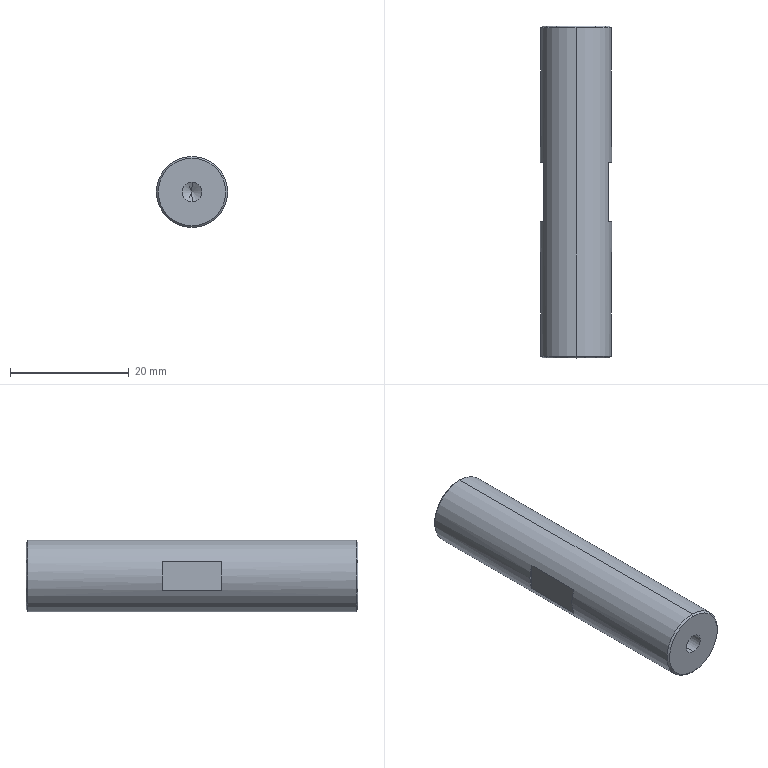Part | STEP file | ND25021-01-JDKM-09B-TL | 1 solid | 22 faces | box 12 x 56 x 12 mm | volume 6119 mm3 | cone 8 | plane 8 | cylinder 6 | commonest cylinder face diameters 3.3 x4 12 x2
STEP:
#1=CARTESIAN_POINT('',(0.,0.,0.));
#2=DIRECTION('',(0.,0.,1.));
#3=DIRECTION('',(1.,0.,0.));
#4=AXIS2_PLACEMENT_3D('',#1,#2,#3);
#5=CARTESIAN_POINT('',(0.,-28.,-5.7));
#6=VERTEX_POINT('',#5);
#7=CARTESIAN_POINT('',(0.,-28.,5.7));
#8=VERTEX_POINT('',#7);
#9=CARTESIAN_POINT('',(0.,-28.,0.));
#10=DIRECTION('',(0.,-1.,0.));
#11=DIRECTION('',(0.,0.,1.));
#12=AXIS2_PLACEMENT_3D('',#9,#10,#11);
#13=CIRCLE('',#12,5.7);
#14=CARTESIAN_POINT('',(0.,-27.7,0.));
#15=DIRECTION('',(0.,1.,0.));
#16=DIRECTION('',(0.,0.,1.));
#17=AXIS2_PLACEMENT_3D('',#14,#15,#16);
#18=CONICAL_SURFACE('',#17,6.,0.7854);
#19=CARTESIAN_POINT('',(6.283,-0.3));
#20=DIRECTION('',(-1.,0.));
#21=VECTOR('',#20,1.);
#22=LINE('',#19,#21);
#23=(GEOMETRIC_REPRESENTATION_CONTEXT(2)PARAMETRIC_REPRESENTATION_CONTEXT()REPRESENTATION_CONTEXT('',''));
#24=DEFINITIONAL_REPRESENTATION('',(#22),#23);
#25=PCURVE('',#18,#24);
#26=CARTESIAN_POINT('',(0.,-28.,0.));
#27=DIRECTION('',(0.,1.,0.));
#28=DIRECTION('',(0.,0.,1.));
#29=AXIS2_PLACEMENT_3D('',#26,#27,#28);
#30=PLANE('',#29);
#31=CARTESIAN_POINT('',(5.7,0.));
#32=CARTESIAN_POINT('',(5.7,-9.873));
#33=CARTESIAN_POINT('',(-2.85,-4.936));
#34=CARTESIAN_POINT('',(-11.4,0.));
#35=CARTESIAN_POINT('',(-2.85,4.936));
#36=CARTESIAN_POINT('',(5.7,9.873));
#37=CARTESIAN_POINT('',(5.7,0.));
#38=(BOUNDED_CURVE()B_SPLINE_CURVE(2,(#31,#32,#33,#34,#35,#36,#37),.UNSPECIFIED.,.T.,.F.)B_SPLINE_CURVE_WITH_KNOTS((1,2,2,2,2,1),(-2.094,0.,2.094,4.189,6.283,8.378),.UNSPECIFIED.)CURVE()GEOMETRIC_REPRESENTATION_ITEM()RATIONAL_B_SPLINE_CURVE((1.,0.5,1.,0.5,1.,0.5,1.))REPRESENTATION_ITEM(''));
#39=(GEOMETRIC_REPRESENTATION_CONTEXT(2)PARAMETRIC_REPRESENTATION_CONTEXT()REPRESENTATION_CONTEXT('',''));
#40=DEFINITIONAL_REPRESENTATION('',(#38),#39);
#41=PCURVE('',#30,#40);
#42=SURFACE_CURVE('',#13,(#25,#41),.PCURVE_S1.);
#43=EDGE_CURVE('',#6,#8,#42,.T.);
#44=ORIENTED_EDGE('',*,*,#43,.F.);
#45=CARTESIAN_POINT('',(0.,-27.7,-6.));
#46=VERTEX_POINT('',#45);
#47=CARTESIAN_POINT('',(0.,-27.7,-6.));
#48=DIRECTION('',(0.,0.7071,-0.7071));
#49=VECTOR('',#48,1.);
#50=LINE('',#47,#49);
#51=CARTESIAN_POINT('',(3.142,0.));
#52=DIRECTION('',(0.,1.));
#53=VECTOR('',#52,1.);
#54=LINE('',#51,#53);
#55=(GEOMETRIC_REPRESENTATION_CONTEXT(2)PARAMETRIC_REPRESENTATION_CONTEXT()REPRESENTATION_CONTEXT('',''));
#56=DEFINITIONAL_REPRESENTATION('',(#54),#55);
#57=PCURVE('',#18,#56);
#58=CARTESIAN_POINT('',(0.,-27.7,0.));
#59=DIRECTION('',(0.,1.,0.));
#60=DIRECTION('',(0.,0.,1.));
#61=AXIS2_PLACEMENT_3D('',#58,#59,#60);
#62=CONICAL_SURFACE('',#61,6.,0.7854);
#63=CARTESIAN_POINT('',(3.142,0.));
#64=DIRECTION('',(0.,1.));
#65=VECTOR('',#64,1.);
#66=LINE('',#63,#65);
#67=(GEOMETRIC_REPRESENTATION_CONTEXT(2)PARAMETRIC_REPRESENTATION_CONTEXT()REPRESENTATION_CONTEXT('',''));
#68=DEFINITIONAL_REPRESENTATION('',(#66),#67);
#69=PCURVE('',#62,#68);
#70=SURFACE_CURVE('',#50,(#57,#69),.PCURVE_S1.);
#71=EDGE_CURVE('',#6,#46,#70,.T.);
#72=ORIENTED_EDGE('',*,*,#71,.T.);
#73=CARTESIAN_POINT('',(0.,-27.7,6.));
#74=VERTEX_POINT('',#73);
#75=CARTESIAN_POINT('',(0.,-27.7,0.));
#76=DIRECTION('',(0.,1.,0.));
#77=DIRECTION('',(0.,0.,1.));
#78=AXIS2_PLACEMENT_3D('',#75,#76,#77);
#79=CIRCLE('',#78,6.);
#80=CARTESIAN_POINT('',(0.,0.));
#81=DIRECTION('',(1.,0.));
#82=VECTOR('',#81,1.);
#83=LINE('',#80,#82);
#84=(GEOMETRIC_REPRESENTATION_CONTEXT(2)PARAMETRIC_REPRESENTATION_CONTEXT()REPRESENTATION_CONTEXT('',''));
#85=DEFINITIONAL_REPRESENTATION('',(#83),#84);
#86=PCURVE('',#18,#85);
#87=CARTESIAN_POINT('',(0.,28.,0.));
#88=DIRECTION('',(0.,-1.,0.));
#89=DIRECTION('',(0.,0.,-1.));
#90=AXIS2_PLACEMENT_3D('',#87,#88,#89);
#91=CYLINDRICAL_SURFACE('',#90,6.);
#92=CARTESIAN_POINT('',(3.142,55.7));
#93=DIRECTION('',(-1.,0.));
#94=VECTOR('',#93,1.);
#95=LINE('',#92,#94);
#96=(GEOMETRIC_REPRESENTATION_CONTEXT(2)PARAMETRIC_REPRESENTATION_CONTEXT()REPRESENTATION_CONTEXT('',''));
#97=DEFINITIONAL_REPRESENTATION('',(#95),#96);
#98=PCURVE('',#91,#97);
#99=SURFACE_CURVE('',#79,(#86,#98),.PCURVE_S1.);
#100=EDGE_CURVE('',#74,#46,#99,.T.);
#101=ORIENTED_EDGE('',*,*,#100,.F.);
#102=CARTESIAN_POINT('',(0.,-27.7,6.));
#103=DIRECTION('',(0.,0.7071,0.7071));
#104=VECTOR('',#103,1.);
#105=LINE('',#102,#104);
#106=CARTESIAN_POINT('',(0.,0.));
#107=DIRECTION('',(0.,1.));
#108=VECTOR('',#107,1.);
#109=LINE('',#106,#108);
#110=(GEOMETRIC_REPRESENTATION_CONTEXT(2)PARAMETRIC_REPRESENTATION_CONTEXT()REPRESENTATION_CONTEXT('',''));
#111=DEFINITIONAL_REPRESENTATION('',(#109),#110);
#112=PCURVE('',#18,#111);
#113=CARTESIAN_POINT('',(6.283,0.));
#114=DIRECTION('',(0.,1.));
#115=VECTOR('',#114,1.);
#116=LINE('',#113,#115);
#117=(GEOMETRIC_REPRESENTATION_CONTEXT(2)PARAMETRIC_REPRESENTATION_CONTEXT()REPRESENTATION_CONTEXT('',''));
#118=DEFINITIONAL_REPRESENTATION('',(#116),#117);
#119=PCURVE('',#62,#118);
#120=SURFACE_CURVE('',#105,(#112,#119),.PCURVE_S1.);
#121=EDGE_CURVE('',#8,#74,#120,.T.);
#122=ORIENTED_EDGE('',*,*,#121,.F.);
#123=EDGE_LOOP('',(#44,#72,#101,#122));
#124=FACE_BOUND('',#123,.T.);
#125=ADVANCED_FACE('',(#124),#18,.T.);
#126=CARTESIAN_POINT('',(0.,28.,5.7));
#127=VERTEX_POINT('',#126);
#128=CARTESIAN_POINT('',(0.,28.,-5.7));
#129=VERTEX_POINT('',#128);
#130=CARTESIAN_POINT('',(0.,28.,0.));
#131=DIRECTION('',(0.,1.,0.));
#132=DIRECTION('',(0.,0.,1.));
#133=AXIS2_PLACEMENT_3D('',#130,#131,#132);
#134=CIRCLE('',#133,5.7);
#135=CARTESIAN_POINT('',(0.,28.,0.));
#136=DIRECTION('',(0.,-1.,0.));
#137=DIRECTION('',(0.,0.,-1.));
#138=AXIS2_PLACEMENT_3D('',#135,#136,#137);
#139=CONICAL_SURFACE('',#138,5.7,0.7854);
#140=CARTESIAN_POINT('',(3.142,0.));
#141=DIRECTION('',(-1.,0.));
#142=VECTOR('',#141,1.);
#143=LINE('',#140,#142);
#144=(GEOMETRIC_REPRESENTATION_CONTEXT(2)PARAMETRIC_REPRESENTATION_CONTEXT()REPRESENTATION_CONTEXT('',''));
#145=DEFINITIONAL_REPRESENTATION('',(#143),#144);
#146=PCURVE('',#139,#145);
#147=CARTESIAN_POINT('',(0.,28.,0.));
#148=DIRECTION('',(0.,1.,0.));
#149=DIRECTION('',(0.,0.,1.));
#150=AXIS2_PLACEMENT_3D('',#147,#148,#149);
#151=PLANE('',#150);
#152=CARTESIAN_POINT('',(0.,0.));
#153=DIRECTION('',(1.,0.));
#154=AXIS2_PLACEMENT_2D('',#152,#153);
#155=CIRCLE('',#154,5.7);
#156=(GEOMETRIC_REPRESENTATION_CONTEXT(2)PARAMETRIC_REPRESENTATION_CONTEXT()REPRESENTATION_CONTEXT('',''));
#157=DEFINITIONAL_REPRESENTATION('',(#155),#156);
#158=PCURVE('',#151,#157);
#159=SURFACE_CURVE('',#134,(#146,#158),.PCURVE_S1.);
#160=EDGE_CURVE('',#127,#129,#159,.T.);
#161=ORIENTED_EDGE('',*,*,#160,.F.);
#162=CARTESIAN_POINT('',(0.,27.7,6.));
#163=VERTEX_POINT('',#162);
#164=CARTESIAN_POINT('',(0.,28.,5.7));
#165=DIRECTION('',(0.,-0.7071,0.7071));
#166=VECTOR('',#165,1.);
#167=LINE('',#164,#166);
#168=CARTESIAN_POINT('',(3.142,0.));
#169=DIRECTION('',(0.,1.));
#170=VECTOR('',#169,1.);
#171=LINE('',#168,#170);
#172=(GEOMETRIC_REPRESENTATION_CONTEXT(2)PARAMETRIC_REPRESENTATION_CONTEXT()REPRESENTATION_CONTEXT('',''));
#173=DEFINITIONAL_REPRESENTATION('',(#171),#172);
#174=PCURVE('',#139,#173);
#175=CARTESIAN_POINT('',(0.,28.,0.));
#176=DIRECTION('',(0.,-1.,0.));
#177=DIRECTION('',(0.,0.,-1.));
#178=AXIS2_PLACEMENT_3D('',#175,#176,#177);
#179=CONICAL_SURFACE('',#178,5.7,0.7854);
#180=CARTESIAN_POINT('',(3.142,0.));
#181=DIRECTION('',(0.,1.));
#182=VECTOR('',#181,1.);
#183=LINE('',#180,#182);
#184=(GEOMETRIC_REPRESENTATION_CONTEXT(2)PARAMETRIC_REPRESENTATION_CONTEXT()REPRESENTATION_CONTEXT('',''));
#185=DEFINITIONAL_REPRESENTATION('',(#183),#184);
#186=PCURVE('',#179,#185);
#187=SURFACE_CURVE('',#167,(#174,#186),.PCURVE_S1.);
#188=EDGE_CURVE('',#127,#163,#187,.T.);
#189=ORIENTED_EDGE('',*,*,#188,.T.);
#190=CARTESIAN_POINT('',(0.,27.7,-6.));
#191=VERTEX_POINT('',#190);
#192=CARTESIAN_POINT('',(0.,27.7,0.));
#193=DIRECTION('',(0.,-1.,0.));
#194=DIRECTION('',(0.,0.,1.));
#195=AXIS2_PLACEMENT_3D('',#192,#193,#194);
#196=CIRCLE('',#195,6.);
#197=CARTESIAN_POINT('',(-3.142,0.3));
#198=DIRECTION('',(1.,0.));
#199=VECTOR('',#198,1.);
#200=LINE('',#197,#199);
#201=(GEOMETRIC_REPRESENTATION_CONTEXT(2)PARAMETRIC_REPRESENTATION_CONTEXT()REPRESENTATION_CONTEXT('',''));
#202=DEFINITIONAL_REPRESENTATION('',(#200),#201);
#203=PCURVE('',#139,#202);
#204=CARTESIAN_POINT('',(-3.142,0.3));
#205=DIRECTION('',(1.,0.));
#206=VECTOR('',#205,1.);
#207=LINE('',#204,#206);
#208=(GEOMETRIC_REPRESENTATION_CONTEXT(2)PARAMETRIC_REPRESENTATION_CONTEXT()REPRESENTATION_CONTEXT('',''));
#209=DEFINITIONAL_REPRESENTATION('',(#207),#208);
#210=PCURVE('',#91,#209);
#211=SURFACE_CURVE('',#196,(#203,#210),.PCURVE_S1.);
#212=EDGE_CURVE('',#191,#163,#211,.T.);
#213=ORIENTED_EDGE('',*,*,#212,.F.);
#214=CARTESIAN_POINT('',(0.,28.,-5.7));
#215=DIRECTION('',(0.,-0.7071,-0.7071));
#216=VECTOR('',#215,1.);
#217=LINE('',#214,#216);
#218=CARTESIAN_POINT('',(0.,0.));
#219=DIRECTION('',(0.,1.));
#220=VECTOR('',#219,1.);
#221=LINE('',#218,#220);
#222=(GEOMETRIC_REPRESENTATION_CONTEXT(2)PARAMETRIC_REPRESENTATION_CONTEXT()REPRESENTATION_CONTEXT('',''));
#223=DEFINITIONAL_REPRESENTATION('',(#221),#222);
#224=PCURVE('',#139,#223);
#225=CARTESIAN_POINT('',(6.283,0.));
#226=DIRECTION('',(0.,1.));
#227=VECTOR('',#226,1.);
#228=LINE('',#225,#227);
#229=(GEOMETRIC_REPRESENTATION_CONTEXT(2)PARAMETRIC_REPRESENTATION_CONTEXT()REPRESENTATION_CONTEXT('',''));
#230=DEFINITIONAL_REPRESENTATION('',(#228),#229);
#231=PCURVE('',#179,#230);
#232=SURFACE_CURVE('',#217,(#224,#231),.PCURVE_S1.);
#233=EDGE_CURVE('',#129,#191,#232,.T.);
#234=ORIENTED_EDGE('',*,*,#233,.F.);
#235=EDGE_LOOP('',(#161,#189,#213,#234));
#236=FACE_BOUND('',#235,.T.);
#237=ADVANCED_FACE('',(#236),#139,.T.);
#238=CARTESIAN_POINT('',(0.,-17.9,-1.65));
#239=VERTEX_POINT('',#238);
#240=CARTESIAN_POINT('',(0.,-28.,-1.65));
#241=VERTEX_POINT('',#240);
#242=CARTESIAN_POINT('',(0.,-28.,-1.65));
#243=DIRECTION('',(0.,-1.,0.));
#244=VECTOR('',#243,1.);
#245=LINE('',#242,#244);
#246=CARTESIAN_POINT('',(0.,-28.,0.));
#247=DIRECTION('',(0.,-1.,0.));
#248=DIRECTION('',(0.,0.,-1.));
#249=AXIS2_PLACEMENT_3D('',#246,#247,#248);
#250=CYLINDRICAL_SURFACE('',#249,1.65);
#251=CARTESIAN_POINT('',(6.283,0.));
#252=DIRECTION('',(0.,1.));
#253=VECTOR('',#252,1.);
#254=LINE('',#251,#253);
#255=(GEOMETRIC_REPRESENTATION_CONTEXT(2)PARAMETRIC_REPRESENTATION_CONTEXT()REPRESENTATION_CONTEXT('',''));
#256=DEFINITIONAL_REPRESENTATION('',(#254),#255);
#257=PCURVE('',#250,#256);
#258=CARTESIAN_POINT('',(0.,-28.,0.));
#259=DIRECTION('',(0.,-1.,0.));
#260=DIRECTION('',(0.,0.,-1.));
#261=AXIS2_PLACEMENT_3D('',#258,#259,#260);
#262=CYLINDRICAL_SURFACE('',#261,1.65);
#263=CARTESIAN_POINT('',(0.,0.));
#264=DIRECTION('',(0.,1.));
#265=VECTOR('',#264,1.);
#266=LINE('',#263,#265);
#267=(GEOMETRIC_REPRESENTATION_CONTEXT(2)PARAMETRIC_REPRESENTATION_CONTEXT()REPRESENTATION_CONTEXT('',''));
#268=DEFINITIONAL_REPRESENTATION('',(#266),#267);
#269=PCURVE('',#262,#268);
#270=SURFACE_CURVE('',#245,(#257,#269),.PCURVE_S1.);
#271=EDGE_CURVE('',#239,#241,#270,.T.);
#272=ORIENTED_EDGE('',*,*,#271,.T.);
#273=CARTESIAN_POINT('',(0.,-28.,1.65));
#274=VERTEX_POINT('',#273);
#275=CARTESIAN_POINT('',(0.,-28.,0.));
#276=DIRECTION('',(0.,-1.,0.));
#277=DIRECTION('',(0.,0.,-1.));
#278=AXIS2_PLACEMENT_3D('',#275,#276,#277);
#279=CIRCLE('',#278,1.65);
#280=CARTESIAN_POINT('',(0.,0.));
#281=DIRECTION('',(1.,0.));
#282=VECTOR('',#281,1.);
#283=LINE('',#280,#282);
#284=(GEOMETRIC_REPRESENTATION_CONTEXT(2)PARAMETRIC_REPRESENTATION_CONTEXT()REPRESENTATION_CONTEXT('',''));
#285=DEFINITIONAL_REPRESENTATION('',(#283),#284);
#286=PCURVE('',#250,#285);
#287=CARTESIAN_POINT('',(-1.65,0.));
#288=CARTESIAN_POINT('',(-1.65,2.858));
#289=CARTESIAN_POINT('',(0.825,1.429));
#290=CARTESIAN_POINT('',(3.3,0.));
#291=CARTESIAN_POINT('',(0.825,-1.429));
#292=CARTESIAN_POINT('',(-1.65,-2.858));
#293=CARTESIAN_POINT('',(-1.65,0.));
#294=(BOUNDED_CURVE()B_SPLINE_CURVE(2,(#287,#288,#289,#290,#291,#292,#293),.UNSPECIFIED.,.T.,.F.)B_SPLINE_CURVE_WITH_KNOTS((1,2,2,2,2,1),(-2.094,0.,2.094,4.189,6.283,8.378),.UNSPECIFIED.)CURVE()GEOMETRIC_REPRESENTATION_ITEM()RATIONAL_B_SPLINE_CURVE((1.,0.5,1.,0.5,1.,0.5,1.))REPRESENTATION_ITEM(''));
#295=(GEOMETRIC_REPRESENTATION_CONTEXT(2)PARAMETRIC_REPRESENTATION_CONTEXT()REPRESENTATION_CONTEXT('',''));
#296=DEFINITIONAL_REPRESENTATION('',(#294),#295);
#297=PCURVE('',#30,#296);
#298=SURFACE_CURVE('',#279,(#286,#297),.PCURVE_S1.);
#299=EDGE_CURVE('',#274,#241,#298,.T.);
#300=ORIENTED_EDGE('',*,*,#299,.F.);
#301=CARTESIAN_POINT('',(0.,-17.9,1.65));
#302=VERTEX_POINT('',#301);
#303=CARTESIAN_POINT('',(0.,-28.,1.65));
#304=DIRECTION('',(0.,-1.,0.));
#305=VECTOR('',#304,1.);
#306=LINE('',#303,#305);
#307=CARTESIAN_POINT('',(3.142,0.));
#308=DIRECTION('',(0.,1.));
#309=VECTOR('',#308,1.);
#310=LINE('',#307,#309);
#311=(GEOMETRIC_REPRESENTATION_CONTEXT(2)PARAMETRIC_REPRESENTATION_CONTEXT()REPRESENTATION_CONTEXT('',''));
#312=DEFINITIONAL_REPRESENTATION('',(#310),#311);
#313=PCURVE('',#250,#312);
#314=CARTESIAN_POINT('',(3.142,0.));
#315=DIRECTION('',(0.,1.));
#316=VECTOR('',#315,1.);
#317=LINE('',#314,#316);
#318=(GEOMETRIC_REPRESENTATION_CONTEXT(2)PARAMETRIC_REPRESENTATION_CONTEXT()REPRESENTATION_CONTEXT('',''));
#319=DEFINITIONAL_REPRESENTATION('',(#317),#318);
#320=PCURVE('',#262,#319);
#321=SURFACE_CURVE('',#306,(#313,#320),.PCURVE_S1.);
#322=EDGE_CURVE('',#302,#274,#321,.T.);
#323=ORIENTED_EDGE('',*,*,#322,.F.);
#324=CARTESIAN_POINT('',(0.,-17.9,0.));
#325=DIRECTION('',(0.,-1.,0.));
#326=DIRECTION('',(0.,0.,-1.));
#327=AXIS2_PLACEMENT_3D('',#324,#325,#326);
#328=CIRCLE('',#327,1.65);
#329=CARTESIAN_POINT('',(0.,-10.1));
#330=DIRECTION('',(1.,0.));
#331=VECTOR('',#330,1.);
#332=LINE('',#329,#331);
#333=(GEOMETRIC_REPRESENTATION_CONTEXT(2)PARAMETRIC_REPRESENTATION_CONTEXT()REPRESENTATION_CONTEXT('',''));
#334=DEFINITIONAL_REPRESENTATION('',(#332),#333);
#335=PCURVE('',#250,#334);
#336=CARTESIAN_POINT('',(0.,-17.9,0.));
#337=DIRECTION('',(0.,-1.,0.));
#338=DIRECTION('',(0.,0.,-1.));
#339=AXIS2_PLACEMENT_3D('',#336,#337,#338);
#340=CONICAL_SURFACE('',#339,1.65,1.03);
#341=CARTESIAN_POINT('',(0.,0.));
#342=DIRECTION('',(1.,0.));
#343=VECTOR('',#342,1.);
#344=LINE('',#341,#343);
#345=(GEOMETRIC_REPRESENTATION_CONTEXT(2)PARAMETRIC_REPRESENTATION_CONTEXT()REPRESENTATION_CONTEXT('',''));
#346=DEFINITIONAL_REPRESENTATION('',(#344),#345);
#347=PCURVE('',#340,#346);
#348=SURFACE_CURVE('',#328,(#335,#347),.PCURVE_S1.);
#349=EDGE_CURVE('',#302,#239,#348,.T.);
#350=ORIENTED_EDGE('',*,*,#349,.T.);
#351=EDGE_LOOP('',(#272,#300,#323,#350));
#352=FACE_BOUND('',#351,.F.);
#353=ADVANCED_FACE('',(#352),#250,.F.);
#354=ORIENTED_EDGE('',*,*,#349,.F.);
#355=CARTESIAN_POINT('',(0.,-16.909,0.));
#356=VERTEX_POINT('',#355);
#357=CARTESIAN_POINT('',(0.,-17.9,1.65));
#358=DIRECTION('',(0.,-0.515,0.8572));
#359=VECTOR('',#358,1.);
#360=LINE('',#357,#359);
#361=CARTESIAN_POINT('',(3.142,-0.9914));
#362=CARTESIAN_POINT('',(3.142,-0.9764));
#363=CARTESIAN_POINT('',(3.142,-0.9464));
#364=CARTESIAN_POINT('',(3.142,-0.9013));
#365=CARTESIAN_POINT('',(3.142,-0.8562));
#366=CARTESIAN_POINT('',(3.142,-0.8112));
#367=CARTESIAN_POINT('',(3.142,-0.7661));
#368=CARTESIAN_POINT('',(3.142,-0.721));
#369=CARTESIAN_POINT('',(3.142,-0.676));
#370=CARTESIAN_POINT('',(3.142,-0.6309));
#371=CARTESIAN_POINT('',(3.142,-0.5858));
#372=CARTESIAN_POINT('',(3.142,-0.5408));
#373=CARTESIAN_POINT('',(3.142,-0.4957));
#374=CARTESIAN_POINT('',(3.142,-0.4506));
#375=CARTESIAN_POINT('',(3.142,-0.4056));
#376=CARTESIAN_POINT('',(3.142,-0.3605));
#377=CARTESIAN_POINT('',(3.142,-0.3155));
#378=CARTESIAN_POINT('',(3.142,-0.2704));
#379=CARTESIAN_POINT('',(3.142,-0.2253));
#380=CARTESIAN_POINT('',(3.142,-0.1803));
#381=CARTESIAN_POINT('',(3.142,-0.1352));
#382=CARTESIAN_POINT('',(3.142,-0.09013));
#383=CARTESIAN_POINT('',(3.142,-0.04506));
#384=CARTESIAN_POINT('',(3.142,-0.01502));
#385=CARTESIAN_POINT('',(3.142,0.));
#386=B_SPLINE_CURVE_WITH_KNOTS('',3,(#361,#362,#363,#364,#365,#366,#367,#368,#369,#370,#371,#372,#373,#374,#375,#376,#377,#378,#379,#380,#381,#382,#383,#384,#385),.UNSPECIFIED.,.F.,.F.,(4,1,1,1,1,1,1,1,1,1,1,1,1,1,1,1,1,1,1,1,1,1,4),(-1.925,-1.837,-1.75,-1.662,-1.575,-1.487,-1.4,-1.312,-1.225,-1.137,-1.05,-0.9625,-0.875,-0.7875,-0.7,-0.6125,-0.525,-0.4375,-0.35,-0.2625,-0.175,-0.0875,0.),.UNSPECIFIED.);
#387=(GEOMETRIC_REPRESENTATION_CONTEXT(2)PARAMETRIC_REPRESENTATION_CONTEXT()REPRESENTATION_CONTEXT('',''));
#388=DEFINITIONAL_REPRESENTATION('',(#386),#387);
#389=PCURVE('',#340,#388);
#390=CARTESIAN_POINT('',(0.,-17.9,0.));
#391=DIRECTION('',(0.,-1.,0.));
#392=DIRECTION('',(0.,0.,-1.));
#393=AXIS2_PLACEMENT_3D('',#390,#391,#392);
#394=CONICAL_SURFACE('',#393,1.65,1.03);
#395=CARTESIAN_POINT('',(3.142,-0.9914));
#396=CARTESIAN_POINT('',(3.142,-0.9764));
#397=CARTESIAN_POINT('',(3.142,-0.9464));
#398=CARTESIAN_POINT('',(3.142,-0.9013));
#399=CARTESIAN_POINT('',(3.142,-0.8562));
#400=CARTESIAN_POINT('',(3.142,-0.8112));
#401=CARTESIAN_POINT('',(3.142,-0.7661));
#402=CARTESIAN_POINT('',(3.142,-0.721));
#403=CARTESIAN_POINT('',(3.142,-0.676));
#404=CARTESIAN_POINT('',(3.142,-0.6309));
#405=CARTESIAN_POINT('',(3.142,-0.5858));
#406=CARTESIAN_POINT('',(3.142,-0.5408));
#407=CARTESIAN_POINT('',(3.142,-0.4957));
#408=CARTESIAN_POINT('',(3.142,-0.4506));
#409=CARTESIAN_POINT('',(3.142,-0.4056));
#410=CARTESIAN_POINT('',(3.142,-0.3605));
#411=CARTESIAN_POINT('',(3.142,-0.3155));
#412=CARTESIAN_POINT('',(3.142,-0.2704));
#413=CARTESIAN_POINT('',(3.142,-0.2253));
#414=CARTESIAN_POINT('',(3.142,-0.1803));
#415=CARTESIAN_POINT('',(3.142,-0.1352));
#416=CARTESIAN_POINT('',(3.142,-0.09013));
#417=CARTESIAN_POINT('',(3.142,-0.04506));
#418=CARTESIAN_POINT('',(3.142,-0.01502));
#419=CARTESIAN_POINT('',(3.142,0.));
#420=B_SPLINE_CURVE_WITH_KNOTS('',3,(#395,#396,#397,#398,#399,#400,#401,#402,#403,#404,#405,#406,#407,#408,#409,#410,#411,#412,#413,#414,#415,#416,#417,#418,#419),.UNSPECIFIED.,.F.,.F.,(4,1,1,1,1,1,1,1,1,1,1,1,1,1,1,1,1,1,1,1,1,1,4),(-1.925,-1.837,-1.75,-1.662,-1.575,-1.487,-1.4,-1.312,-1.225,-1.137,-1.05,-0.9625,-0.875,-0.7875,-0.7,-0.6125,-0.525,-0.4375,-0.35,-0.2625,-0.175,-0.0875,0.),.UNSPECIFIED.);
#421=(GEOMETRIC_REPRESENTATION_CONTEXT(2)PARAMETRIC_REPRESENTATION_CONTEXT()REPRESENTATION_CONTEXT('',''));
#422=DEFINITIONAL_REPRESENTATION('',(#420),#421);
#423=PCURVE('',#394,#422);
#424=SURFACE_CURVE('',#360,(#389,#423),.PCURVE_S1.);
#425=EDGE_CURVE('',#356,#302,#424,.T.);
#426=ORIENTED_EDGE('',*,*,#425,.F.);
#427=CARTESIAN_POINT('',(0.,-17.9,-1.65));
#428=DIRECTION('',(0.,-0.515,-0.8572));
#429=VECTOR('',#428,1.);
#430=LINE('',#427,#429);
#431=CARTESIAN_POINT('',(6.283,-0.9914));
#432=CARTESIAN_POINT('',(6.283,-0.9764));
#433=CARTESIAN_POINT('',(6.283,-0.9464));
#434=CARTESIAN_POINT('',(6.283,-0.9013));
#435=CARTESIAN_POINT('',(6.283,-0.8562));
#436=CARTESIAN_POINT('',(6.283,-0.8112));
#437=CARTESIAN_POINT('',(6.283,-0.7661));
#438=CARTESIAN_POINT('',(6.283,-0.721));
#439=CARTESIAN_POINT('',(6.283,-0.676));
#440=CARTESIAN_POINT('',(6.283,-0.6309));
#441=CARTESIAN_POINT('',(6.283,-0.5858));
#442=CARTESIAN_POINT('',(6.283,-0.5408));
#443=CARTESIAN_POINT('',(6.283,-0.4957));
#444=CARTESIAN_POINT('',(6.283,-0.4506));
#445=CARTESIAN_POINT('',(6.283,-0.4056));
#446=CARTESIAN_POINT('',(6.283,-0.3605));
#447=CARTESIAN_POINT('',(6.283,-0.3155));
#448=CARTESIAN_POINT('',(6.283,-0.2704));
#449=CARTESIAN_POINT('',(6.283,-0.2253));
#450=CARTESIAN_POINT('',(6.283,-0.1803));
#451=CARTESIAN_POINT('',(6.283,-0.1352));
#452=CARTESIAN_POINT('',(6.283,-0.09013));
#453=CARTESIAN_POINT('',(6.283,-0.04506));
#454=CARTESIAN_POINT('',(6.283,-0.01502));
#455=CARTESIAN_POINT('',(6.283,0.));
#456=B_SPLINE_CURVE_WITH_KNOTS('',3,(#431,#432,#433,#434,#435,#436,#437,#438,#439,#440,#441,#442,#443,#444,#445,#446,#447,#448,#449,#450,#451,#452,#453,#454,#455),.UNSPECIFIED.,.F.,.F.,(4,1,1,1,1,1,1,1,1,1,1,1,1,1,1,1,1,1,1,1,1,1,4),(-1.925,-1.837,-1.75,-1.662,-1.575,-1.487,-1.4,-1.312,-1.225,-1.137,-1.05,-0.9625,-0.875,-0.7875,-0.7,-0.6125,-0.525,-0.4375,-0.35,-0.2625,-0.175,-0.0875,0.),.UNSPECIFIED.);
#457=(GEOMETRIC_REPRESENTATION_CONTEXT(2)PARAMETRIC_REPRESENTATION_CONTEXT()REPRESENTATION_CONTEXT('',''));
#458=DEFINITIONAL_REPRESENTATION('',(#456),#457);
#459=PCURVE('',#340,#458);
#460=CARTESIAN_POINT('',(0.,-0.9914));
#461=CARTESIAN_POINT('',(0.,-0.9764));
#462=CARTESIAN_POINT('',(0.,-0.9464));
#463=CARTESIAN_POINT('',(0.,-0.9013));
#464=CARTESIAN_POINT('',(0.,-0.8562));
#465=CARTESIAN_POINT('',(0.,-0.8112));
#466=CARTESIAN_POINT('',(0.,-0.7661));
#467=CARTESIAN_POINT('',(0.,-0.721));
#468=CARTESIAN_POINT('',(0.,-0.676));
#469=CARTESIAN_POINT('',(0.,-0.6309));
#470=CARTESIAN_POINT('',(0.,-0.5858));
#471=CARTESIAN_POINT('',(0.,-0.5408));
#472=CARTESIAN_POINT('',(0.,-0.4957));
#473=CARTESIAN_POINT('',(0.,-0.4506));
#474=CARTESIAN_POINT('',(0.,-0.4056));
#475=CARTESIAN_POINT('',(0.,-0.3605));
#476=CARTESIAN_POINT('',(0.,-0.3155));
#477=CARTESIAN_POINT('',(0.,-0.2704));
#478=CARTESIAN_POINT('',(0.,-0.2253));
#479=CARTESIAN_POINT('',(0.,-0.1803));
#480=CARTESIAN_POINT('',(0.,-0.1352));
#481=CARTESIAN_POINT('',(0.,-0.09013));
#482=CARTESIAN_POINT('',(0.,-0.04506));
#483=CARTESIAN_POINT('',(0.,-0.01502));
#484=CARTESIAN_POINT('',(0.,0.));
#485=B_SPLINE_CURVE_WITH_KNOTS('',3,(#460,#461,#462,#463,#464,#465,#466,#467,#468,#469,#470,#471,#472,#473,#474,#475,#476,#477,#478,#479,#480,#481,#482,#483,#484),.UNSPECIFIED.,.F.,.F.,(4,1,1,1,1,1,1,1,1,1,1,1,1,1,1,1,1,1,1,1,1,1,4),(-1.925,-1.837,-1.75,-1.662,-1.575,-1.487,-1.4,-1.312,-1.225,-1.137,-1.05,-0.9625,-0.875,-0.7875,-0.7,-0.6125,-0.525,-0.4375,-0.35,-0.2625,-0.175,-0.0875,0.),.UNSPECIFIED.);
#486=(GEOMETRIC_REPRESENTATION_CONTEXT(2)PARAMETRIC_REPRESENTATION_CONTEXT()REPRESENTATION_CONTEXT('',''));
#487=DEFINITIONAL_REPRESENTATION('',(#485),#486);
#488=PCURVE('',#394,#487);
#489=SURFACE_CURVE('',#430,(#459,#488),.PCURVE_S1.);
#490=EDGE_CURVE('',#356,#239,#489,.T.);
#491=ORIENTED_EDGE('',*,*,#490,.T.);
#492=EDGE_LOOP('',(#354,#426,#491));
#493=FACE_BOUND('',#492,.F.);
#494=ADVANCED_FACE('',(#493),#340,.F.);
#495=CARTESIAN_POINT('',(0.,17.9,1.65));
#496=VERTEX_POINT('',#495);
#497=CARTESIAN_POINT('',(0.,28.,1.65));
#498=VERTEX_POINT('',#497);
#499=CARTESIAN_POINT('',(0.,28.,1.65));
#500=DIRECTION('',(0.,1.,0.));
#501=VECTOR('',#500,1.);
#502=LINE('',#499,#501);
#503=CARTESIAN_POINT('',(0.,28.,0.));
#504=DIRECTION('',(0.,1.,0.));
#505=DIRECTION('',(0.,0.,1.));
#506=AXIS2_PLACEMENT_3D('',#503,#504,#505);
#507=CYLINDRICAL_SURFACE('',#506,1.65);
#508=CARTESIAN_POINT('',(6.283,0.));
#509=DIRECTION('',(0.,1.));
#510=VECTOR('',#509,1.);
#511=LINE('',#508,#510);
#512=(GEOMETRIC_REPRESENTATION_CONTEXT(2)PARAMETRIC_REPRESENTATION_CONTEXT()REPRESENTATION_CONTEXT('',''));
#513=DEFINITIONAL_REPRESENTATION('',(#511),#512);
#514=PCURVE('',#507,#513);
#515=CARTESIAN_POINT('',(0.,28.,0.));
#516=DIRECTION('',(0.,1.,0.));
#517=DIRECTION('',(0.,0.,1.));
#518=AXIS2_PLACEMENT_3D('',#515,#516,#517);
#519=CYLINDRICAL_SURFACE('',#518,1.65);
#520=CARTESIAN_POINT('',(0.,0.));
#521=DIRECTION('',(0.,1.));
#522=VECTOR('',#521,1.);
#523=LINE('',#520,#522);
#524=(GEOMETRIC_REPRESENTATION_CONTEXT(2)PARAMETRIC_REPRESENTATION_CONTEXT()REPRESENTATION_CONTEXT('',''));
#525=DEFINITIONAL_REPRESENTATION('',(#523),#524);
#526=PCURVE('',#519,#525);
#527=SURFACE_CURVE('',#502,(#514,#526),.PCURVE_S1.);
#528=EDGE_CURVE('',#496,#498,#527,.T.);
#529=ORIENTED_EDGE('',*,*,#528,.T.);
#530=CARTESIAN_POINT('',(0.,28.,-1.65));
#531=VERTEX_POINT('',#530);
#532=CARTESIAN_POINT('',(0.,28.,0.));
#533=DIRECTION('',(0.,1.,0.));
#534=DIRECTION('',(0.,0.,1.));
#535=AXIS2_PLACEMENT_3D('',#532,#533,#534);
#536=CIRCLE('',#535,1.65);
#537=CARTESIAN_POINT('',(0.,0.));
#538=DIRECTION('',(1.,0.));
#539=VECTOR('',#538,1.);
#540=LINE('',#537,#539);
#541=(GEOMETRIC_REPRESENTATION_CONTEXT(2)PARAMETRIC_REPRESENTATION_CONTEXT()REPRESENTATION_CONTEXT('',''));
#542=DEFINITIONAL_REPRESENTATION('',(#540),#541);
#543=PCURVE('',#507,#542);
#544=CARTESIAN_POINT('',(0.,0.));
#545=DIRECTION('',(1.,0.));
#546=AXIS2_PLACEMENT_2D('',#544,#545);
#547=CIRCLE('',#546,1.65);
#548=(GEOMETRIC_REPRESENTATION_CONTEXT(2)PARAMETRIC_REPRESENTATION_CONTEXT()REPRESENTATION_CONTEXT('',''));
#549=DEFINITIONAL_REPRESENTATION('',(#547),#548);
#550=PCURVE('',#151,#549);
#551=SURFACE_CURVE('',#536,(#543,#550),.PCURVE_S1.);
#552=EDGE_CURVE('',#531,#498,#551,.T.);
#553=ORIENTED_EDGE('',*,*,#552,.F.);
#554=CARTESIAN_POINT('',(0.,17.9,-1.65));
#555=VERTEX_POINT('',#554);
#556=CARTESIAN_POINT('',(0.,28.,-1.65));
#557=DIRECTION('',(0.,1.,0.));
#558=VECTOR('',#557,1.);
#559=LINE('',#556,#558);
#560=CARTESIAN_POINT('',(3.142,0.));
#561=DIRECTION('',(0.,1.));
#562=VECTOR('',#561,1.);
#563=LINE('',#560,#562);
#564=(GEOMETRIC_REPRESENTATION_CONTEXT(2)PARAMETRIC_REPRESENTATION_CONTEXT()REPRESENTATION_CONTEXT('',''));
#565=DEFINITIONAL_REPRESENTATION('',(#563),#564);
#566=PCURVE('',#507,#565);
#567=CARTESIAN_POINT('',(3.142,0.));
#568=DIRECTION('',(0.,1.));
#569=VECTOR('',#568,1.);
#570=LINE('',#567,#569);
#571=(GEOMETRIC_REPRESENTATION_CONTEXT(2)PARAMETRIC_REPRESENTATION_CONTEXT()REPRESENTATION_CONTEXT('',''));
#572=DEFINITIONAL_REPRESENTATION('',(#570),#571);
#573=PCURVE('',#519,#572);
#574=SURFACE_CURVE('',#559,(#566,#573),.PCURVE_S1.);
#575=EDGE_CURVE('',#555,#531,#574,.T.);
#576=ORIENTED_EDGE('',*,*,#575,.F.);
#577=CARTESIAN_POINT('',(0.,17.9,0.));
#578=DIRECTION('',(0.,1.,0.));
#579=DIRECTION('',(0.,0.,1.));
#580=AXIS2_PLACEMENT_3D('',#577,#578,#579);
#581=CIRCLE('',#580,1.65);
#582=CARTESIAN_POINT('',(0.,-10.1));
#583=DIRECTION('',(1.,0.));
#584=VECTOR('',#583,1.);
#585=LINE('',#582,#584);
#586=(GEOMETRIC_REPRESENTATION_CONTEXT(2)PARAMETRIC_REPRESENTATION_CONTEXT()REPRESENTATION_CONTEXT('',''));
#587=DEFINITIONAL_REPRESENTATION('',(#585),#586);
#588=PCURVE('',#507,#587);
#589=CARTESIAN_POINT('',(0.,17.9,0.));
#590=DIRECTION('',(0.,1.,0.));
#591=DIRECTION('',(0.,0.,1.));
#592=AXIS2_PLACEMENT_3D('',#589,#590,#591);
#593=CONICAL_SURFACE('',#592,1.65,1.03);
#594=CARTESIAN_POINT('',(0.,0.));
#595=DIRECTION('',(1.,0.));
#596=VECTOR('',#595,1.);
#597=LINE('',#594,#596);
#598=(GEOMETRIC_REPRESENTATION_CONTEXT(2)PARAMETRIC_REPRESENTATION_CONTEXT()REPRESENTATION_CONTEXT('',''));
#599=DEFINITIONAL_REPRESENTATION('',(#597),#598);
#600=PCURVE('',#593,#599);
#601=SURFACE_CURVE('',#581,(#588,#600),.PCURVE_S1.);
#602=EDGE_CURVE('',#555,#496,#601,.T.);
#603=ORIENTED_EDGE('',*,*,#602,.T.);
#604=EDGE_LOOP('',(#529,#553,#576,#603));
#605=FACE_BOUND('',#604,.F.);
#606=ADVANCED_FACE('',(#605),#507,.F.);
#607=ORIENTED_EDGE('',*,*,#602,.F.);
#608=CARTESIAN_POINT('',(0.,16.909,0.));
#609=VERTEX_POINT('',#608);
#610=CARTESIAN_POINT('',(0.,17.9,-1.65));
#611=DIRECTION('',(0.,0.515,-0.8572));
#612=VECTOR('',#611,1.);
#613=LINE('',#610,#612);
#614=CARTESIAN_POINT('',(3.142,0.));
#615=DIRECTION('',(0.,1.));
#616=VECTOR('',#615,1.);
#617=LINE('',#614,#616);
#618=(GEOMETRIC_REPRESENTATION_CONTEXT(2)PARAMETRIC_REPRESENTATION_CONTEXT()REPRESENTATION_CONTEXT('',''));
#619=DEFINITIONAL_REPRESENTATION('',(#617),#618);
#620=PCURVE('',#593,#619);
#621=CARTESIAN_POINT('',(0.,17.9,0.));
#622=DIRECTION('',(0.,1.,0.));
#623=DIRECTION('',(0.,0.,1.));
#624=AXIS2_PLACEMENT_3D('',#621,#622,#623);
#625=CONICAL_SURFACE('',#624,1.65,1.03);
#626=CARTESIAN_POINT('',(3.142,0.));
#627=DIRECTION('',(0.,1.));
#628=VECTOR('',#627,1.);
#629=LINE('',#626,#628);
#630=(GEOMETRIC_REPRESENTATION_CONTEXT(2)PARAMETRIC_REPRESENTATION_CONTEXT()REPRESENTATION_CONTEXT('',''));
#631=DEFINITIONAL_REPRESENTATION('',(#629),#630);
#632=PCURVE('',#625,#631);
#633=SURFACE_CURVE('',#613,(#620,#632),.PCURVE_S1.);
#634=EDGE_CURVE('',#609,#555,#633,.T.);
#635=ORIENTED_EDGE('',*,*,#634,.F.);
#636=CARTESIAN_POINT('',(0.,17.9,1.65));
#637=DIRECTION('',(0.,0.515,0.8572));
#638=VECTOR('',#637,1.);
#639=LINE('',#636,#638);
#640=CARTESIAN_POINT('',(6.283,0.));
#641=DIRECTION('',(0.,1.));
#642=VECTOR('',#641,1.);
#643=LINE('',#640,#642);
#644=(GEOMETRIC_REPRESENTATION_CONTEXT(2)PARAMETRIC_REPRESENTATION_CONTEXT()REPRESENTATION_CONTEXT('',''));
#645=DEFINITIONAL_REPRESENTATION('',(#643),#644);
#646=PCURVE('',#593,#645);
#647=CARTESIAN_POINT('',(0.,0.));
#648=DIRECTION('',(0.,1.));
#649=VECTOR('',#648,1.);
#650=LINE('',#647,#649);
#651=(GEOMETRIC_REPRESENTATION_CONTEXT(2)PARAMETRIC_REPRESENTATION_CONTEXT()REPRESENTATION_CONTEXT('',''));
#652=DEFINITIONAL_REPRESENTATION('',(#650),#651);
#653=PCURVE('',#625,#652);
#654=SURFACE_CURVE('',#639,(#646,#653),.PCURVE_S1.);
#655=EDGE_CURVE('',#609,#496,#654,.T.);
#656=ORIENTED_EDGE('',*,*,#655,.T.);
#657=EDGE_LOOP('',(#607,#635,#656));
#658=FACE_BOUND('',#657,.F.);
#659=ADVANCED_FACE('',(#658),#593,.F.);
#660=CARTESIAN_POINT('',(5.5,5.,-2.398));
#661=VERTEX_POINT('',#660);
#662=CARTESIAN_POINT('',(5.5,-5.,-2.398));
#663=VERTEX_POINT('',#662);
#664=CARTESIAN_POINT('',(5.5,28.,-2.398));
#665=DIRECTION('',(0.,-1.,0.));
#666=VECTOR('',#665,1.);
#667=LINE('',#664,#666);
#668=CARTESIAN_POINT('',(1.16,0.));
#669=DIRECTION('',(0.,1.));
#670=VECTOR('',#669,1.);
#671=LINE('',#668,#670);
#672=(GEOMETRIC_REPRESENTATION_CONTEXT(2)PARAMETRIC_REPRESENTATION_CONTEXT()REPRESENTATION_CONTEXT('',''));
#673=DEFINITIONAL_REPRESENTATION('',(#671),#672);
#674=PCURVE('',#91,#673);
#675=CARTESIAN_POINT('',(5.5,5.,-5.));
#676=DIRECTION('',(-1.,0.,0.));
#677=DIRECTION('',(0.,0.,1.));
#678=AXIS2_PLACEMENT_3D('',#675,#676,#677);
#679=PLANE('',#678);
#680=CARTESIAN_POINT('',(2.602,23.));
#681=DIRECTION('',(0.,-1.));
#682=VECTOR('',#681,1.);
#683=LINE('',#680,#682);
#684=(GEOMETRIC_REPRESENTATION_CONTEXT(2)PARAMETRIC_REPRESENTATION_CONTEXT()REPRESENTATION_CONTEXT('',''));
#685=DEFINITIONAL_REPRESENTATION('',(#683),#684);
#686=PCURVE('',#679,#685);
#687=SURFACE_CURVE('',#667,(#674,#686),.PCURVE_S1.);
#688=EDGE_CURVE('',#661,#663,#687,.T.);
#689=ORIENTED_EDGE('',*,*,#688,.T.);
#690=CARTESIAN_POINT('',(5.5,-5.,2.398));
#691=VERTEX_POINT('',#690);
#692=CARTESIAN_POINT('',(0.,-5.,0.));
#693=DIRECTION('',(0.,-1.,0.));
#694=DIRECTION('',(0.,0.,-1.));
#695=AXIS2_PLACEMENT_3D('',#692,#693,#694);
#696=CIRCLE('',#695,6.);
#697=CARTESIAN_POINT('',(0.,33.));
#698=DIRECTION('',(1.,0.));
#699=VECTOR('',#698,1.);
#700=LINE('',#697,#699);
#701=(GEOMETRIC_REPRESENTATION_CONTEXT(2)PARAMETRIC_REPRESENTATION_CONTEXT()REPRESENTATION_CONTEXT('',''));
#702=DEFINITIONAL_REPRESENTATION('',(#700),#701);
#703=PCURVE('',#91,#702);
#704=CARTESIAN_POINT('',(6.,-5.,-5.));
#705=DIRECTION('',(0.,-1.,0.));
#706=DIRECTION('',(0.,0.,-1.));
#707=AXIS2_PLACEMENT_3D('',#704,#705,#706);
#708=PLANE('',#707);
#709=CARTESIAN_POINT('',(-5.,-6.));
#710=DIRECTION('',(1.,0.));
#711=AXIS2_PLACEMENT_2D('',#709,#710);
#712=CIRCLE('',#711,6.);
#713=(GEOMETRIC_REPRESENTATION_CONTEXT(2)PARAMETRIC_REPRESENTATION_CONTEXT()REPRESENTATION_CONTEXT('',''));
#714=DEFINITIONAL_REPRESENTATION('',(#712),#713);
#715=PCURVE('',#708,#714);
#716=SURFACE_CURVE('',#696,(#703,#715),.PCURVE_S1.);
#717=EDGE_CURVE('',#663,#691,#716,.T.);
#718=ORIENTED_EDGE('',*,*,#717,.T.);
#719=CARTESIAN_POINT('',(5.5,5.,2.398));
#720=VERTEX_POINT('',#719);
#721=CARTESIAN_POINT('',(5.5,28.,2.398));
#722=DIRECTION('',(0.,1.,0.));
#723=VECTOR('',#722,1.);
#724=LINE('',#721,#723);
#725=CARTESIAN_POINT('',(1.982,0.));
#726=DIRECTION('',(0.,-1.));
#727=VECTOR('',#726,1.);
#728=LINE('',#725,#727);
#729=(GEOMETRIC_REPRESENTATION_CONTEXT(2)PARAMETRIC_REPRESENTATION_CONTEXT()REPRESENTATION_CONTEXT('',''));
#730=DEFINITIONAL_REPRESENTATION('',(#728),#729);
#731=PCURVE('',#91,#730);
#732=CARTESIAN_POINT('',(7.398,23.));
#733=DIRECTION('',(0.,1.));
#734=VECTOR('',#733,1.);
#735=LINE('',#732,#734);
#736=(GEOMETRIC_REPRESENTATION_CONTEXT(2)PARAMETRIC_REPRESENTATION_CONTEXT()REPRESENTATION_CONTEXT('',''));
#737=DEFINITIONAL_REPRESENTATION('',(#735),#736);
#738=PCURVE('',#679,#737);
#739=SURFACE_CURVE('',#724,(#731,#738),.PCURVE_S1.);
#740=EDGE_CURVE('',#691,#720,#739,.T.);
#741=ORIENTED_EDGE('',*,*,#740,.T.);
#742=CARTESIAN_POINT('',(0.,5.,0.));
#743=DIRECTION('',(0.,1.,0.));
#744=DIRECTION('',(0.,0.,1.));
#745=AXIS2_PLACEMENT_3D('',#742,#743,#744);
#746=CIRCLE('',#745,6.);
#747=CARTESIAN_POINT('',(3.142,23.));
#748=DIRECTION('',(-1.,0.));
#749=VECTOR('',#748,1.);
#750=LINE('',#747,#749);
#751=(GEOMETRIC_REPRESENTATION_CONTEXT(2)PARAMETRIC_REPRESENTATION_CONTEXT()REPRESENTATION_CONTEXT('',''));
#752=DEFINITIONAL_REPRESENTATION('',(#750),#751);
#753=PCURVE('',#91,#752);
#754=CARTESIAN_POINT('',(6.,5.,-5.));
#755=DIRECTION('',(0.,1.,0.));
#756=DIRECTION('',(0.,0.,1.));
#757=AXIS2_PLACEMENT_3D('',#754,#755,#756);
#758=PLANE('',#757);
#759=CARTESIAN_POINT('',(5.,-6.));
#760=DIRECTION('',(1.,0.));
#761=AXIS2_PLACEMENT_2D('',#759,#760);
#762=CIRCLE('',#761,6.);
#763=(GEOMETRIC_REPRESENTATION_CONTEXT(2)PARAMETRIC_REPRESENTATION_CONTEXT()REPRESENTATION_CONTEXT('',''));
#764=DEFINITIONAL_REPRESENTATION('',(#762),#763);
#765=PCURVE('',#758,#764);
#766=SURFACE_CURVE('',#746,(#753,#765),.PCURVE_S1.);
#767=EDGE_CURVE('',#720,#661,#766,.T.);
#768=ORIENTED_EDGE('',*,*,#767,.T.);
#769=EDGE_LOOP('',(#689,#718,#741,#768));
#770=FACE_BOUND('',#769,.T.);
#771=ORIENTED_EDGE('',*,*,#212,.T.);
#772=CARTESIAN_POINT('',(0.,28.,6.));
#773=DIRECTION('',(0.,-1.,0.));
#774=VECTOR('',#773,1.);
#775=LINE('',#772,#774);
#776=CARTESIAN_POINT('',(3.142,0.));
#777=DIRECTION('',(0.,1.));
#778=VECTOR('',#777,1.);
#779=LINE('',#776,#778);
#780=(GEOMETRIC_REPRESENTATION_CONTEXT(2)PARAMETRIC_REPRESENTATION_CONTEXT()REPRESENTATION_CONTEXT('',''));
#781=DEFINITIONAL_REPRESENTATION('',(#779),#780);
#782=PCURVE('',#91,#781);
#783=CARTESIAN_POINT('',(0.,28.,0.));
#784=DIRECTION('',(0.,-1.,0.));
#785=DIRECTION('',(0.,0.,-1.));
#786=AXIS2_PLACEMENT_3D('',#783,#784,#785);
#787=CYLINDRICAL_SURFACE('',#786,6.);
#788=CARTESIAN_POINT('',(3.142,0.));
#789=DIRECTION('',(0.,1.));
#790=VECTOR('',#789,1.);
#791=LINE('',#788,#790);
#792=(GEOMETRIC_REPRESENTATION_CONTEXT(2)PARAMETRIC_REPRESENTATION_CONTEXT()REPRESENTATION_CONTEXT('',''));
#793=DEFINITIONAL_REPRESENTATION('',(#791),#792);
#794=PCURVE('',#787,#793);
#795=SURFACE_CURVE('',#775,(#782,#794),.PCURVE_S1.);
#796=EDGE_CURVE('',#163,#74,#795,.T.);
#797=ORIENTED_EDGE('',*,*,#796,.T.);
#798=ORIENTED_EDGE('',*,*,#100,.T.);
#799=CARTESIAN_POINT('',(0.,28.,-6.));
#800=DIRECTION('',(0.,-1.,0.));
#801=VECTOR('',#800,1.);
#802=LINE('',#799,#801);
#803=CARTESIAN_POINT('',(0.,0.));
#804=DIRECTION('',(0.,1.));
#805=VECTOR('',#804,1.);
#806=LINE('',#803,#805);
#807=(GEOMETRIC_REPRESENTATION_CONTEXT(2)PARAMETRIC_REPRESENTATION_CONTEXT()REPRESENTATION_CONTEXT('',''));
#808=DEFINITIONAL_REPRESENTATION('',(#806),#807);
#809=PCURVE('',#91,#808);
#810=CARTESIAN_POINT('',(6.283,0.));
#811=DIRECTION('',(0.,1.));
#812=VECTOR('',#811,1.);
#813=LINE('',#810,#812);
#814=(GEOMETRIC_REPRESENTATION_CONTEXT(2)PARAMETRIC_REPRESENTATION_CONTEXT()REPRESENTATION_CONTEXT('',''));
#815=DEFINITIONAL_REPRESENTATION('',(#813),#814);
#816=PCURVE('',#787,#815);
#817=SURFACE_CURVE('',#802,(#809,#816),.PCURVE_S1.);
#818=EDGE_CURVE('',#191,#46,#817,.T.);
#819=ORIENTED_EDGE('',*,*,#818,.F.);
#820=EDGE_LOOP('',(#771,#797,#798,#819));
#821=FACE_BOUND('',#820,.T.);
#822=ADVANCED_FACE('',(#770,#821),#91,.T.);
#823=ORIENTED_EDGE('',*,*,#796,.F.);
#824=CARTESIAN_POINT('',(0.,27.7,0.));
#825=DIRECTION('',(0.,-1.,0.));
#826=DIRECTION('',(0.,0.,1.));
#827=AXIS2_PLACEMENT_3D('',#824,#825,#826);
#828=CIRCLE('',#827,6.);
#829=CARTESIAN_POINT('',(3.142,0.3));
#830=DIRECTION('',(1.,0.));
#831=VECTOR('',#830,1.);
#832=LINE('',#829,#831);
#833=(GEOMETRIC_REPRESENTATION_CONTEXT(2)PARAMETRIC_REPRESENTATION_CONTEXT()REPRESENTATION_CONTEXT('',''));
#834=DEFINITIONAL_REPRESENTATION('',(#832),#833);
#835=PCURVE('',#787,#834);
#836=CARTESIAN_POINT('',(3.142,0.3));
#837=DIRECTION('',(1.,0.));
#838=VECTOR('',#837,1.);
#839=LINE('',#836,#838);
#840=(GEOMETRIC_REPRESENTATION_CONTEXT(2)PARAMETRIC_REPRESENTATION_CONTEXT()REPRESENTATION_CONTEXT('',''));
#841=DEFINITIONAL_REPRESENTATION('',(#839),#840);
#842=PCURVE('',#179,#841);
#843=SURFACE_CURVE('',#828,(#835,#842),.PCURVE_S1.);
#844=EDGE_CURVE('',#163,#191,#843,.T.);
#845=ORIENTED_EDGE('',*,*,#844,.T.);
#846=ORIENTED_EDGE('',*,*,#818,.T.);
#847=CARTESIAN_POINT('',(0.,-27.7,0.));
#848=DIRECTION('',(0.,1.,0.));
#849=DIRECTION('',(0.,0.,1.));
#850=AXIS2_PLACEMENT_3D('',#847,#848,#849);
#851=CIRCLE('',#850,6.);
#852=CARTESIAN_POINT('',(9.425,55.7));
#853=DIRECTION('',(-1.,0.));
#854=VECTOR('',#853,1.);
#855=LINE('',#852,#854);
#856=(GEOMETRIC_REPRESENTATION_CONTEXT(2)PARAMETRIC_REPRESENTATION_CONTEXT()REPRESENTATION_CONTEXT('',''));
#857=DEFINITIONAL_REPRESENTATION('',(#855),#856);
#858=PCURVE('',#787,#857);
#859=CARTESIAN_POINT('',(0.,0.));
#860=DIRECTION('',(1.,0.));
#861=VECTOR('',#860,1.);
#862=LINE('',#859,#861);
#863=(GEOMETRIC_REPRESENTATION_CONTEXT(2)PARAMETRIC_REPRESENTATION_CONTEXT()REPRESENTATION_CONTEXT('',''));
#864=DEFINITIONAL_REPRESENTATION('',(#862),#863);
#865=PCURVE('',#62,#864);
#866=SURFACE_CURVE('',#851,(#858,#865),.PCURVE_S1.);
#867=EDGE_CURVE('',#46,#74,#866,.T.);
#868=ORIENTED_EDGE('',*,*,#867,.T.);
#869=EDGE_LOOP('',(#823,#845,#846,#868));
#870=FACE_BOUND('',#869,.T.);
#871=CARTESIAN_POINT('',(-5.5,5.,2.398));
#872=VERTEX_POINT('',#871);
#873=CARTESIAN_POINT('',(-5.5,-5.,2.398));
#874=VERTEX_POINT('',#873);
#875=CARTESIAN_POINT('',(-5.5,28.,2.398));
#876=DIRECTION('',(0.,-1.,0.));
#877=VECTOR('',#876,1.);
#878=LINE('',#875,#877);
#879=CARTESIAN_POINT('',(4.301,0.));
#880=DIRECTION('',(0.,1.));
#881=VECTOR('',#880,1.);
#882=LINE('',#879,#881);
#883=(GEOMETRIC_REPRESENTATION_CONTEXT(2)PARAMETRIC_REPRESENTATION_CONTEXT()REPRESENTATION_CONTEXT('',''));
#884=DEFINITIONAL_REPRESENTATION('',(#882),#883);
#885=PCURVE('',#787,#884);
#886=CARTESIAN_POINT('',(-5.5,5.,-5.));
#887=DIRECTION('',(1.,0.,0.));
#888=DIRECTION('',(0.,0.,-1.));
#889=AXIS2_PLACEMENT_3D('',#886,#887,#888);
#890=PLANE('',#889);
#891=CARTESIAN_POINT('',(-7.398,23.));
#892=DIRECTION('',(0.,-1.));
#893=VECTOR('',#892,1.);
#894=LINE('',#891,#893);
#895=(GEOMETRIC_REPRESENTATION_CONTEXT(2)PARAMETRIC_REPRESENTATION_CONTEXT()REPRESENTATION_CONTEXT('',''));
#896=DEFINITIONAL_REPRESENTATION('',(#894),#895);
#897=PCURVE('',#890,#896);
#898=SURFACE_CURVE('',#878,(#885,#897),.PCURVE_S1.);
#899=EDGE_CURVE('',#872,#874,#898,.T.);
#900=ORIENTED_EDGE('',*,*,#899,.T.);
#901=CARTESIAN_POINT('',(-5.5,-5.,-2.398));
#902=VERTEX_POINT('',#901);
#903=CARTESIAN_POINT('',(0.,-5.,0.));
#904=DIRECTION('',(0.,-1.,0.));
#905=DIRECTION('',(0.,0.,-1.));
#906=AXIS2_PLACEMENT_3D('',#903,#904,#905);
#907=CIRCLE('',#906,6.);
#908=CARTESIAN_POINT('',(0.,33.));
#909=DIRECTION('',(1.,0.));
#910=VECTOR('',#909,1.);
#911=LINE('',#908,#910);
#912=(GEOMETRIC_REPRESENTATION_CONTEXT(2)PARAMETRIC_REPRESENTATION_CONTEXT()REPRESENTATION_CONTEXT('',''));
#913=DEFINITIONAL_REPRESENTATION('',(#911),#912);
#914=PCURVE('',#787,#913);
#915=CARTESIAN_POINT('',(-6.,-5.,-5.));
#916=DIRECTION('',(0.,-1.,0.));
#917=DIRECTION('',(0.,0.,-1.));
#918=AXIS2_PLACEMENT_3D('',#915,#916,#917);
#919=PLANE('',#918);
#920=CARTESIAN_POINT('',(-5.,6.));
#921=DIRECTION('',(1.,0.));
#922=AXIS2_PLACEMENT_2D('',#920,#921);
#923=CIRCLE('',#922,6.);
#924=(GEOMETRIC_REPRESENTATION_CONTEXT(2)PARAMETRIC_REPRESENTATION_CONTEXT()REPRESENTATION_CONTEXT('',''));
#925=DEFINITIONAL_REPRESENTATION('',(#923),#924);
#926=PCURVE('',#919,#925);
#927=SURFACE_CURVE('',#907,(#914,#926),.PCURVE_S1.);
#928=EDGE_CURVE('',#874,#902,#927,.T.);
#929=ORIENTED_EDGE('',*,*,#928,.T.);
#930=CARTESIAN_POINT('',(-5.5,5.,-2.398));
#931=VERTEX_POINT('',#930);
#932=CARTESIAN_POINT('',(-5.5,28.,-2.398));
#933=DIRECTION('',(0.,1.,0.));
#934=VECTOR('',#933,1.);
#935=LINE('',#932,#934);
#936=CARTESIAN_POINT('',(5.124,0.));
#937=DIRECTION('',(0.,-1.));
#938=VECTOR('',#937,1.);
#939=LINE('',#936,#938);
#940=(GEOMETRIC_REPRESENTATION_CONTEXT(2)PARAMETRIC_REPRESENTATION_CONTEXT()REPRESENTATION_CONTEXT('',''));
#941=DEFINITIONAL_REPRESENTATION('',(#939),#940);
#942=PCURVE('',#787,#941);
#943=CARTESIAN_POINT('',(-2.602,23.));
#944=DIRECTION('',(0.,1.));
#945=VECTOR('',#944,1.);
#946=LINE('',#943,#945);
#947=(GEOMETRIC_REPRESENTATION_CONTEXT(2)PARAMETRIC_REPRESENTATION_CONTEXT()REPRESENTATION_CONTEXT('',''));
#948=DEFINITIONAL_REPRESENTATION('',(#946),#947);
#949=PCURVE('',#890,#948);
#950=SURFACE_CURVE('',#935,(#942,#949),.PCURVE_S1.);
#951=EDGE_CURVE('',#902,#931,#950,.T.);
#952=ORIENTED_EDGE('',*,*,#951,.T.);
#953=CARTESIAN_POINT('',(0.,5.,0.));
#954=DIRECTION('',(0.,1.,0.));
#955=DIRECTION('',(0.,0.,1.));
#956=AXIS2_PLACEMENT_3D('',#953,#954,#955);
#957=CIRCLE('',#956,6.);
#958=CARTESIAN_POINT('',(9.425,23.));
#959=DIRECTION('',(-1.,0.));
#960=VECTOR('',#959,1.);
#961=LINE('',#958,#960);
#962=(GEOMETRIC_REPRESENTATION_CONTEXT(2)PARAMETRIC_REPRESENTATION_CONTEXT()REPRESENTATION_CONTEXT('',''));
#963=DEFINITIONAL_REPRESENTATION('',(#961),#962);
#964=PCURVE('',#787,#963);
#965=CARTESIAN_POINT('',(-6.,5.,-5.));
#966=DIRECTION('',(0.,1.,0.));
#967=DIRECTION('',(0.,0.,1.));
#968=AXIS2_PLACEMENT_3D('',#965,#966,#967);
#969=PLANE('',#968);
#970=CARTESIAN_POINT('',(5.,6.));
#971=DIRECTION('',(1.,0.));
#972=AXIS2_PLACEMENT_2D('',#970,#971);
#973=CIRCLE('',#972,6.);
#974=(GEOMETRIC_REPRESENTATION_CONTEXT(2)PARAMETRIC_REPRESENTATION_CONTEXT()REPRESENTATION_CONTEXT('',''));
#975=DEFINITIONAL_REPRESENTATION('',(#973),#974);
#976=PCURVE('',#969,#975);
#977=SURFACE_CURVE('',#957,(#964,#976),.PCURVE_S1.);
#978=EDGE_CURVE('',#931,#872,#977,.T.);
#979=ORIENTED_EDGE('',*,*,#978,.T.);
#980=EDGE_LOOP('',(#900,#929,#952,#979));
#981=FACE_BOUND('',#980,.T.);
#982=ADVANCED_FACE('',(#870,#981),#787,.T.);
#983=CARTESIAN_POINT('',(0.,28.,0.));
#984=DIRECTION('',(0.,1.,0.));
#985=DIRECTION('',(0.,0.,1.));
#986=AXIS2_PLACEMENT_3D('',#983,#984,#985);
#987=CIRCLE('',#986,5.7);
#988=CARTESIAN_POINT('',(0.,0.));
#989=DIRECTION('',(1.,0.));
#990=AXIS2_PLACEMENT_2D('',#988,#989);
#991=CIRCLE('',#990,5.7);
#992=(GEOMETRIC_REPRESENTATION_CONTEXT(2)PARAMETRIC_REPRESENTATION_CONTEXT()REPRESENTATION_CONTEXT('',''));
#993=DEFINITIONAL_REPRESENTATION('',(#991),#992);
#994=PCURVE('',#151,#993);
#995=CARTESIAN_POINT('',(9.425,0.));
#996=DIRECTION('',(-1.,0.));
#997=VECTOR('',#996,1.);
#998=LINE('',#995,#997);
#999=(GEOMETRIC_REPRESENTATION_CONTEXT(2)PARAMETRIC_REPRESENTATION_CONTEXT()REPRESENTATION_CONTEXT('',''));
#1000=DEFINITIONAL_REPRESENTATION('',(#998),#999);
#1001=PCURVE('',#179,#1000);
#1002=SURFACE_CURVE('',#987,(#994,#1001),.PCURVE_S1.);
#1003=EDGE_CURVE('',#129,#127,#1002,.T.);
#1004=ORIENTED_EDGE('',*,*,#1003,.T.);
#1005=ORIENTED_EDGE('',*,*,#160,.T.);
#1006=EDGE_LOOP('',(#1004,#1005));
#1007=FACE_BOUND('',#1006,.T.);
#1008=CARTESIAN_POINT('',(0.,28.,0.));
#1009=DIRECTION('',(0.,1.,0.));
#1010=DIRECTION('',(0.,0.,1.));
#1011=AXIS2_PLACEMENT_3D('',#1008,#1009,#1010);
#1012=CIRCLE('',#1011,1.65);
#1013=CARTESIAN_POINT('',(0.,0.));
#1014=DIRECTION('',(1.,0.));
#1015=AXIS2_PLACEMENT_2D('',#1013,#1014);
#1016=CIRCLE('',#1015,1.65);
#1017=(GEOMETRIC_REPRESENTATION_CONTEXT(2)PARAMETRIC_REPRESENTATION_CONTEXT()REPRESENTATION_CONTEXT('',''));
#1018=DEFINITIONAL_REPRESENTATION('',(#1016),#1017);
#1019=PCURVE('',#151,#1018);
#1020=CARTESIAN_POINT('',(0.,0.));
#1021=DIRECTION('',(1.,0.));
#1022=VECTOR('',#1021,1.);
#1023=LINE('',#1020,#1022);
#1024=(GEOMETRIC_REPRESENTATION_CONTEXT(2)PARAMETRIC_REPRESENTATION_CONTEXT()REPRESENTATION_CONTEXT('',''));
#1025=DEFINITIONAL_REPRESENTATION('',(#1023),#1024);
#1026=PCURVE('',#519,#1025);
#1027=SURFACE_CURVE('',#1012,(#1019,#1026),.PCURVE_S1.);
#1028=EDGE_CURVE('',#498,#531,#1027,.T.);
#1029=ORIENTED_EDGE('',*,*,#1028,.F.);
#1030=ORIENTED_EDGE('',*,*,#552,.F.);
#1031=EDGE_LOOP('',(#1029,#1030));
#1032=FACE_BOUND('',#1031,.T.);
#1033=ADVANCED_FACE('',(#1007,#1032),#151,.T.);
#1034=CARTESIAN_POINT('',(0.,-28.,0.));
#1035=DIRECTION('',(0.,-1.,0.));
#1036=DIRECTION('',(0.,0.,1.));
#1037=AXIS2_PLACEMENT_3D('',#1034,#1035,#1036);
#1038=CIRCLE('',#1037,5.7);
#1039=CARTESIAN_POINT('',(5.7,0.));
#1040=CARTESIAN_POINT('',(5.7,-9.873));
#1041=CARTESIAN_POINT('',(-2.85,-4.936));
#1042=CARTESIAN_POINT('',(-11.4,0.));
#1043=CARTESIAN_POINT('',(-2.85,4.936));
#1044=CARTESIAN_POINT('',(5.7,9.873));
#1045=CARTESIAN_POINT('',(5.7,0.));
#1046=(BOUNDED_CURVE()B_SPLINE_CURVE(2,(#1039,#1040,#1041,#1042,#1043,#1044,#1045),.UNSPECIFIED.,.T.,.F.)B_SPLINE_CURVE_WITH_KNOTS((1,2,2,2,2,1),(-2.094,0.,2.094,4.189,6.283,8.378),.UNSPECIFIED.)CURVE()GEOMETRIC_REPRESENTATION_ITEM()RATIONAL_B_SPLINE_CURVE((1.,0.5,1.,0.5,1.,0.5,1.))REPRESENTATION_ITEM(''));
#1047=(GEOMETRIC_REPRESENTATION_CONTEXT(2)PARAMETRIC_REPRESENTATION_CONTEXT()REPRESENTATION_CONTEXT('',''));
#1048=DEFINITIONAL_REPRESENTATION('',(#1046),#1047);
#1049=PCURVE('',#30,#1048);
#1050=CARTESIAN_POINT('',(6.283,-0.3));
#1051=DIRECTION('',(-1.,0.));
#1052=VECTOR('',#1051,1.);
#1053=LINE('',#1050,#1052);
#1054=(GEOMETRIC_REPRESENTATION_CONTEXT(2)PARAMETRIC_REPRESENTATION_CONTEXT()REPRESENTATION_CONTEXT('',''));
#1055=DEFINITIONAL_REPRESENTATION('',(#1053),#1054);
#1056=PCURVE('',#62,#1055);
#1057=SURFACE_CURVE('',#1038,(#1049,#1056),.PCURVE_S1.);
#1058=EDGE_CURVE('',#8,#6,#1057,.T.);
#1059=ORIENTED_EDGE('',*,*,#1058,.T.);
#1060=ORIENTED_EDGE('',*,*,#43,.T.);
#1061=EDGE_LOOP('',(#1059,#1060));
#1062=FACE_BOUND('',#1061,.T.);
#1063=CARTESIAN_POINT('',(0.,-28.,0.));
#1064=DIRECTION('',(0.,-1.,0.));
#1065=DIRECTION('',(0.,0.,-1.));
#1066=AXIS2_PLACEMENT_3D('',#1063,#1064,#1065);
#1067=CIRCLE('',#1066,1.65);
#1068=CARTESIAN_POINT('',(-1.65,0.));
#1069=CARTESIAN_POINT('',(-1.65,2.858));
#1070=CARTESIAN_POINT('',(0.825,1.429));
#1071=CARTESIAN_POINT('',(3.3,0.));
#1072=CARTESIAN_POINT('',(0.825,-1.429));
#1073=CARTESIAN_POINT('',(-1.65,-2.858));
#1074=CARTESIAN_POINT('',(-1.65,0.));
#1075=(BOUNDED_CURVE()B_SPLINE_CURVE(2,(#1068,#1069,#1070,#1071,#1072,#1073,#1074),.UNSPECIFIED.,.T.,.F.)B_SPLINE_CURVE_WITH_KNOTS((1,2,2,2,2,1),(-2.094,0.,2.094,4.189,6.283,8.378),.UNSPECIFIED.)CURVE()GEOMETRIC_REPRESENTATION_ITEM()RATIONAL_B_SPLINE_CURVE((1.,0.5,1.,0.5,1.,0.5,1.))REPRESENTATION_ITEM(''));
#1076=(GEOMETRIC_REPRESENTATION_CONTEXT(2)PARAMETRIC_REPRESENTATION_CONTEXT()REPRESENTATION_CONTEXT('',''));
#1077=DEFINITIONAL_REPRESENTATION('',(#1075),#1076);
#1078=PCURVE('',#30,#1077);
#1079=CARTESIAN_POINT('',(0.,0.));
#1080=DIRECTION('',(1.,0.));
#1081=VECTOR('',#1080,1.);
#1082=LINE('',#1079,#1081);
#1083=(GEOMETRIC_REPRESENTATION_CONTEXT(2)PARAMETRIC_REPRESENTATION_CONTEXT()REPRESENTATION_CONTEXT('',''));
#1084=DEFINITIONAL_REPRESENTATION('',(#1082),#1083);
#1085=PCURVE('',#262,#1084);
#1086=SURFACE_CURVE('',#1067,(#1078,#1085),.PCURVE_S1.);
#1087=EDGE_CURVE('',#241,#274,#1086,.T.);
#1088=ORIENTED_EDGE('',*,*,#1087,.F.);
#1089=ORIENTED_EDGE('',*,*,#299,.F.);
#1090=EDGE_LOOP('',(#1088,#1089));
#1091=FACE_BOUND('',#1090,.T.);
#1092=ADVANCED_FACE('',(#1062,#1091),#30,.F.);
#1093=CARTESIAN_POINT('',(0.,17.9,0.));
#1094=DIRECTION('',(0.,1.,0.));
#1095=DIRECTION('',(0.,0.,1.));
#1096=AXIS2_PLACEMENT_3D('',#1093,#1094,#1095);
#1097=CIRCLE('',#1096,1.65);
#1098=CARTESIAN_POINT('',(0.,0.));
#1099=DIRECTION('',(1.,0.));
#1100=VECTOR('',#1099,1.);
#1101=LINE('',#1098,#1100);
#1102=(GEOMETRIC_REPRESENTATION_CONTEXT(2)PARAMETRIC_REPRESENTATION_CONTEXT()REPRESENTATION_CONTEXT('',''));
#1103=DEFINITIONAL_REPRESENTATION('',(#1101),#1102);
#1104=PCURVE('',#625,#1103);
#1105=CARTESIAN_POINT('',(0.,-10.1));
#1106=DIRECTION('',(1.,0.));
#1107=VECTOR('',#1106,1.);
#1108=LINE('',#1105,#1107);
#1109=(GEOMETRIC_REPRESENTATION_CONTEXT(2)PARAMETRIC_REPRESENTATION_CONTEXT()REPRESENTATION_CONTEXT('',''));
#1110=DEFINITIONAL_REPRESENTATION('',(#1108),#1109);
#1111=PCURVE('',#519,#1110);
#1112=SURFACE_CURVE('',#1097,(#1104,#1111),.PCURVE_S1.);
#1113=EDGE_CURVE('',#496,#555,#1112,.T.);
#1114=ORIENTED_EDGE('',*,*,#1113,.F.);
#1115=ORIENTED_EDGE('',*,*,#655,.F.);
#1116=ORIENTED_EDGE('',*,*,#634,.T.);
#1117=EDGE_LOOP('',(#1114,#1115,#1116));
#1118=FACE_BOUND('',#1117,.F.);
#1119=ADVANCED_FACE('',(#1118),#625,.F.);
#1120=ORIENTED_EDGE('',*,*,#1028,.F.);
#1121=ORIENTED_EDGE('',*,*,#528,.F.);
#1122=ORIENTED_EDGE('',*,*,#1113,.T.);
#1123=ORIENTED_EDGE('',*,*,#575,.T.);
#1124=EDGE_LOOP('',(#1120,#1121,#1122,#1123));
#1125=FACE_BOUND('',#1124,.F.);
#1126=ADVANCED_FACE('',(#1125),#519,.F.);
#1127=CARTESIAN_POINT('',(0.,-17.9,0.));
#1128=DIRECTION('',(0.,-1.,0.));
#1129=DIRECTION('',(0.,0.,-1.));
#1130=AXIS2_PLACEMENT_3D('',#1127,#1128,#1129);
#1131=CIRCLE('',#1130,1.65);
#1132=CARTESIAN_POINT('',(0.,0.));
#1133=DIRECTION('',(1.,0.));
#1134=VECTOR('',#1133,1.);
#1135=LINE('',#1132,#1134);
#1136=(GEOMETRIC_REPRESENTATION_CONTEXT(2)PARAMETRIC_REPRESENTATION_CONTEXT()REPRESENTATION_CONTEXT('',''));
#1137=DEFINITIONAL_REPRESENTATION('',(#1135),#1136);
#1138=PCURVE('',#394,#1137);
#1139=CARTESIAN_POINT('',(0.,-10.1));
#1140=DIRECTION('',(1.,0.));
#1141=VECTOR('',#1140,1.);
#1142=LINE('',#1139,#1141);
#1143=(GEOMETRIC_REPRESENTATION_CONTEXT(2)PARAMETRIC_REPRESENTATION_CONTEXT()REPRESENTATION_CONTEXT('',''));
#1144=DEFINITIONAL_REPRESENTATION('',(#1142),#1143);
#1145=PCURVE('',#262,#1144);
#1146=SURFACE_CURVE('',#1131,(#1138,#1145),.PCURVE_S1.);
#1147=EDGE_CURVE('',#239,#302,#1146,.T.);
#1148=ORIENTED_EDGE('',*,*,#1147,.F.);
#1149=ORIENTED_EDGE('',*,*,#490,.F.);
#1150=ORIENTED_EDGE('',*,*,#425,.T.);
#1151=EDGE_LOOP('',(#1148,#1149,#1150));
#1152=FACE_BOUND('',#1151,.F.);
#1153=ADVANCED_FACE('',(#1152),#394,.F.);
#1154=ORIENTED_EDGE('',*,*,#1087,.F.);
#1155=ORIENTED_EDGE('',*,*,#271,.F.);
#1156=ORIENTED_EDGE('',*,*,#1147,.T.);
#1157=ORIENTED_EDGE('',*,*,#322,.T.);
#1158=EDGE_LOOP('',(#1154,#1155,#1156,#1157));
#1159=FACE_BOUND('',#1158,.F.);
#1160=ADVANCED_FACE('',(#1159),#262,.F.);
#1161=ORIENTED_EDGE('',*,*,#188,.F.);
#1162=ORIENTED_EDGE('',*,*,#1003,.F.);
#1163=ORIENTED_EDGE('',*,*,#233,.T.);
#1164=ORIENTED_EDGE('',*,*,#844,.F.);
#1165=EDGE_LOOP('',(#1161,#1162,#1163,#1164));
#1166=FACE_BOUND('',#1165,.T.);
#1167=ADVANCED_FACE('',(#1166),#179,.T.);
#1168=ORIENTED_EDGE('',*,*,#71,.F.);
#1169=ORIENTED_EDGE('',*,*,#1058,.F.);
#1170=ORIENTED_EDGE('',*,*,#121,.T.);
#1171=ORIENTED_EDGE('',*,*,#867,.F.);
#1172=EDGE_LOOP('',(#1168,#1169,#1170,#1171));
#1173=FACE_BOUND('',#1172,.T.);
#1174=ADVANCED_FACE('',(#1173),#62,.T.);
#1175=CARTESIAN_POINT('',(-5.5,5.,-5.));
#1176=DIRECTION('',(0.,0.,1.));
#1177=VECTOR('',#1176,1.);
#1178=LINE('',#1175,#1177);
#1179=CARTESIAN_POINT('',(0.,0.5));
#1180=DIRECTION('',(1.,0.));
#1181=VECTOR('',#1180,1.);
#1182=LINE('',#1179,#1181);
#1183=(GEOMETRIC_REPRESENTATION_CONTEXT(2)PARAMETRIC_REPRESENTATION_CONTEXT()REPRESENTATION_CONTEXT('',''));
#1184=DEFINITIONAL_REPRESENTATION('',(#1182),#1183);
#1185=PCURVE('',#969,#1184);
#1186=CARTESIAN_POINT('',(0.,0.));
#1187=DIRECTION('',(-1.,0.));
#1188=VECTOR('',#1187,1.);
#1189=LINE('',#1186,#1188);
#1190=(GEOMETRIC_REPRESENTATION_CONTEXT(2)PARAMETRIC_REPRESENTATION_CONTEXT()REPRESENTATION_CONTEXT('',''));
#1191=DEFINITIONAL_REPRESENTATION('',(#1189),#1190);
#1192=PCURVE('',#890,#1191);
#1193=SURFACE_CURVE('',#1178,(#1185,#1192),.PCURVE_S1.);
#1194=EDGE_CURVE('',#931,#872,#1193,.T.);
#1195=ORIENTED_EDGE('',*,*,#1194,.T.);
#1196=ORIENTED_EDGE('',*,*,#978,.F.);
#1197=EDGE_LOOP('',(#1195,#1196));
#1198=FACE_BOUND('',#1197,.T.);
#1199=ADVANCED_FACE('',(#1198),#969,.F.);
#1200=ORIENTED_EDGE('',*,*,#1194,.F.);
#1201=ORIENTED_EDGE('',*,*,#951,.F.);
#1202=CARTESIAN_POINT('',(-5.5,-5.,-5.));
#1203=DIRECTION('',(0.,0.,1.));
#1204=VECTOR('',#1203,1.);
#1205=LINE('',#1202,#1204);
#1206=CARTESIAN_POINT('',(0.,-10.));
#1207=DIRECTION('',(-1.,0.));
#1208=VECTOR('',#1207,1.);
#1209=LINE('',#1206,#1208);
#1210=(GEOMETRIC_REPRESENTATION_CONTEXT(2)PARAMETRIC_REPRESENTATION_CONTEXT()REPRESENTATION_CONTEXT('',''));
#1211=DEFINITIONAL_REPRESENTATION('',(#1209),#1210);
#1212=PCURVE('',#890,#1211);
#1213=CARTESIAN_POINT('',(0.,0.5));
#1214=DIRECTION('',(-1.,0.));
#1215=VECTOR('',#1214,1.);
#1216=LINE('',#1213,#1215);
#1217=(GEOMETRIC_REPRESENTATION_CONTEXT(2)PARAMETRIC_REPRESENTATION_CONTEXT()REPRESENTATION_CONTEXT('',''));
#1218=DEFINITIONAL_REPRESENTATION('',(#1216),#1217);
#1219=PCURVE('',#919,#1218);
#1220=SURFACE_CURVE('',#1205,(#1212,#1219),.PCURVE_S1.);
#1221=EDGE_CURVE('',#902,#874,#1220,.T.);
#1222=ORIENTED_EDGE('',*,*,#1221,.T.);
#1223=ORIENTED_EDGE('',*,*,#899,.F.);
#1224=EDGE_LOOP('',(#1200,#1201,#1222,#1223));
#1225=FACE_BOUND('',#1224,.T.);
#1226=ADVANCED_FACE('',(#1225),#890,.F.);
#1227=ORIENTED_EDGE('',*,*,#1221,.F.);
#1228=ORIENTED_EDGE('',*,*,#928,.F.);
#1229=EDGE_LOOP('',(#1227,#1228));
#1230=FACE_BOUND('',#1229,.T.);
#1231=ADVANCED_FACE('',(#1230),#919,.F.);
#1232=CARTESIAN_POINT('',(5.5,-5.,-5.));
#1233=DIRECTION('',(0.,0.,1.));
#1234=VECTOR('',#1233,1.);
#1235=LINE('',#1232,#1234);
#1236=CARTESIAN_POINT('',(0.,-0.5));
#1237=DIRECTION('',(-1.,0.));
#1238=VECTOR('',#1237,1.);
#1239=LINE('',#1236,#1238);
#1240=(GEOMETRIC_REPRESENTATION_CONTEXT(2)PARAMETRIC_REPRESENTATION_CONTEXT()REPRESENTATION_CONTEXT('',''));
#1241=DEFINITIONAL_REPRESENTATION('',(#1239),#1240);
#1242=PCURVE('',#708,#1241);
#1243=CARTESIAN_POINT('',(0.,-10.));
#1244=DIRECTION('',(1.,0.));
#1245=VECTOR('',#1244,1.);
#1246=LINE('',#1243,#1245);
#1247=(GEOMETRIC_REPRESENTATION_CONTEXT(2)PARAMETRIC_REPRESENTATION_CONTEXT()REPRESENTATION_CONTEXT('',''));
#1248=DEFINITIONAL_REPRESENTATION('',(#1246),#1247);
#1249=PCURVE('',#679,#1248);
#1250=SURFACE_CURVE('',#1235,(#1242,#1249),.PCURVE_S1.);
#1251=EDGE_CURVE('',#663,#691,#1250,.T.);
#1252=ORIENTED_EDGE('',*,*,#1251,.T.);
#1253=ORIENTED_EDGE('',*,*,#717,.F.);
#1254=EDGE_LOOP('',(#1252,#1253));
#1255=FACE_BOUND('',#1254,.T.);
#1256=ADVANCED_FACE('',(#1255),#708,.F.);
#1257=CARTESIAN_POINT('',(5.5,5.,-5.));
#1258=DIRECTION('',(0.,0.,1.));
#1259=VECTOR('',#1258,1.);
#1260=LINE('',#1257,#1259);
#1261=CARTESIAN_POINT('',(0.,0.));
#1262=DIRECTION('',(1.,0.));
#1263=VECTOR('',#1262,1.);
#1264=LINE('',#1261,#1263);
#1265=(GEOMETRIC_REPRESENTATION_CONTEXT(2)PARAMETRIC_REPRESENTATION_CONTEXT()REPRESENTATION_CONTEXT('',''));
#1266=DEFINITIONAL_REPRESENTATION('',(#1264),#1265);
#1267=PCURVE('',#679,#1266);
#1268=CARTESIAN_POINT('',(0.,-0.5));
#1269=DIRECTION('',(1.,0.));
#1270=VECTOR('',#1269,1.);
#1271=LINE('',#1268,#1270);
#1272=(GEOMETRIC_REPRESENTATION_CONTEXT(2)PARAMETRIC_REPRESENTATION_CONTEXT()REPRESENTATION_CONTEXT('',''));
#1273=DEFINITIONAL_REPRESENTATION('',(#1271),#1272);
#1274=PCURVE('',#758,#1273);
#1275=SURFACE_CURVE('',#1260,(#1267,#1274),.PCURVE_S1.);
#1276=EDGE_CURVE('',#661,#720,#1275,.T.);
#1277=ORIENTED_EDGE('',*,*,#1276,.T.);
#1278=ORIENTED_EDGE('',*,*,#740,.F.);
#1279=ORIENTED_EDGE('',*,*,#1251,.F.);
#1280=ORIENTED_EDGE('',*,*,#688,.F.);
#1281=EDGE_LOOP('',(#1277,#1278,#1279,#1280));
#1282=FACE_BOUND('',#1281,.T.);
#1283=ADVANCED_FACE('',(#1282),#679,.F.);
#1284=ORIENTED_EDGE('',*,*,#1276,.F.);
#1285=ORIENTED_EDGE('',*,*,#767,.F.);
#1286=EDGE_LOOP('',(#1284,#1285));
#1287=FACE_BOUND('',#1286,.T.);
#1288=ADVANCED_FACE('',(#1287),#758,.F.);
#1289=CLOSED_SHELL('',(#125,#237,#353,#494,#606,#659,#822,#982,#1033,#1092,#1119,#1126,#1153,#1160,#1167,#1174,#1199,#1226,#1231,#1256,#1283,#1288));
#1290=MANIFOLD_SOLID_BREP('',#1289);
#1291=(LENGTH_UNIT()NAMED_UNIT(*)SI_UNIT(.MILLI.,.METRE.));
#1292=UNCERTAINTY_MEASURE_WITH_UNIT(LENGTH_MEASURE(0.0000001),#1291,'','');
#1293=(NAMED_UNIT(*)PLANE_ANGLE_UNIT()SI_UNIT($,.RADIAN.));
#1294=(NAMED_UNIT(*)SI_UNIT($,.STERADIAN.)SOLID_ANGLE_UNIT());
#1295=(GEOMETRIC_REPRESENTATION_CONTEXT(3)GLOBAL_UNCERTAINTY_ASSIGNED_CONTEXT((#1292))GLOBAL_UNIT_ASSIGNED_CONTEXT((#1291,#1293,#1294))REPRESENTATION_CONTEXT('',''));
#1296=ADVANCED_BREP_SHAPE_REPRESENTATION('',(#4,#1290),#1295);